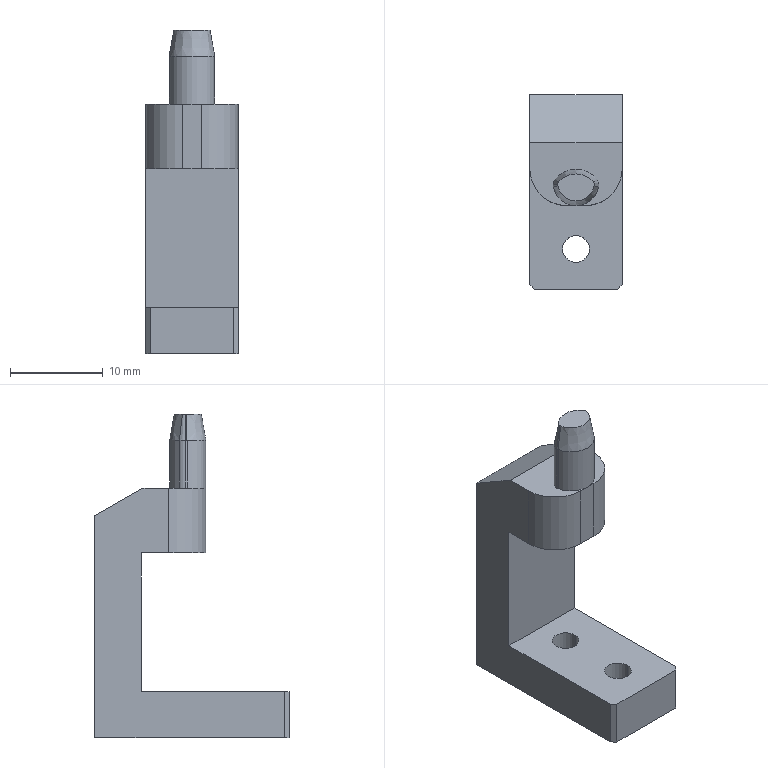Part | SolidWorks | features ICE 4, Chamfer 3, Fillet 2, Extrusion 1, HoleWzd 1 | 1 solid | 36 faces | box 10 x 21 x 35 mm | volume 2531 mm3 | plane 16 | cylinder 15 | cone 5 | commonest cylinder face diameters 2.9 x4 4 x4 2 x3 8 x2 5 x1 5.831 x1
STEP:
#1=CARTESIAN_POINT('',(2.,-11.65,-7.9));
#2=VERTEX_POINT('',#1);
#3=CARTESIAN_POINT('',(-2.,-11.65,-7.9));
#4=VERTEX_POINT('',#3);
#5=CARTESIAN_POINT('',(0.,-11.65,-7.9));
#6=DIRECTION('',(0.,0.,-1.));
#7=DIRECTION('',(-1.,0.,0.));
#8=AXIS2_PLACEMENT_3D('',#5,#6,#7);
#9=CIRCLE('',#8,2.);
#10=EDGE_CURVE('',#2,#4,#9,.T.);
#11=ORIENTED_EDGE('',*,*,#10,.F.);
#12=CARTESIAN_POINT('',(2.,-11.65,-10.));
#13=VERTEX_POINT('',#12);
#14=CARTESIAN_POINT('',(2.,-11.65,-7.9));
#15=DIRECTION('',(0.,0.,-1.));
#16=VECTOR('',#15,1000.);
#17=LINE('',#14,#16);
#18=EDGE_CURVE('',#2,#13,#17,.T.);
#19=ORIENTED_EDGE('',*,*,#18,.T.);
#20=CARTESIAN_POINT('',(-2.,-11.65,-10.));
#21=VERTEX_POINT('',#20);
#22=CARTESIAN_POINT('',(0.,-11.65,-10.));
#23=DIRECTION('',(0.,0.,-1.));
#24=DIRECTION('',(-1.,0.,0.));
#25=AXIS2_PLACEMENT_3D('',#22,#23,#24);
#26=CIRCLE('',#25,2.);
#27=EDGE_CURVE('',#13,#21,#26,.T.);
#28=ORIENTED_EDGE('',*,*,#27,.T.);
#29=CARTESIAN_POINT('',(-2.,-11.65,-7.9));
#30=DIRECTION('',(0.,0.,-1.));
#31=VECTOR('',#30,1000.);
#32=LINE('',#29,#31);
#33=EDGE_CURVE('',#4,#21,#32,.T.);
#34=ORIENTED_EDGE('',*,*,#33,.F.);
#35=EDGE_LOOP('',(#11,#19,#28,#34));
#36=FACE_OUTER_BOUND('',#35,.T.);
#37=CARTESIAN_POINT('',(0.,-11.65,-7.9));
#38=DIRECTION('',(0.,0.,-1.));
#39=DIRECTION('',(-1.,0.,0.));
#40=AXIS2_PLACEMENT_3D('',#37,#38,#39);
#41=CYLINDRICAL_SURFACE('',#40,2.);
#42=ADVANCED_FACE('',(#36),#41,.F.);
#43=CARTESIAN_POINT('',(2.,-3.65,-7.9));
#44=VERTEX_POINT('',#43);
#45=CARTESIAN_POINT('',(-2.,-3.65,-7.9));
#46=VERTEX_POINT('',#45);
#47=CARTESIAN_POINT('',(0.,-3.65,-7.9));
#48=DIRECTION('',(0.,0.,-1.));
#49=DIRECTION('',(-1.,0.,0.));
#50=AXIS2_PLACEMENT_3D('',#47,#48,#49);
#51=CIRCLE('',#50,2.);
#52=EDGE_CURVE('',#44,#46,#51,.T.);
#53=ORIENTED_EDGE('',*,*,#52,.F.);
#54=CARTESIAN_POINT('',(2.,-3.65,-10.));
#55=VERTEX_POINT('',#54);
#56=CARTESIAN_POINT('',(2.,-3.65,-7.9));
#57=DIRECTION('',(0.,0.,-1.));
#58=VECTOR('',#57,1000.);
#59=LINE('',#56,#58);
#60=EDGE_CURVE('',#44,#55,#59,.T.);
#61=ORIENTED_EDGE('',*,*,#60,.T.);
#62=CARTESIAN_POINT('',(-2.,-3.65,-10.));
#63=VERTEX_POINT('',#62);
#64=CARTESIAN_POINT('',(0.,-3.65,-10.));
#65=DIRECTION('',(0.,0.,-1.));
#66=DIRECTION('',(-1.,0.,0.));
#67=AXIS2_PLACEMENT_3D('',#64,#65,#66);
#68=CIRCLE('',#67,2.);
#69=EDGE_CURVE('',#55,#63,#68,.T.);
#70=ORIENTED_EDGE('',*,*,#69,.T.);
#71=CARTESIAN_POINT('',(-2.,-3.65,-7.9));
#72=DIRECTION('',(0.,0.,-1.));
#73=VECTOR('',#72,1000.);
#74=LINE('',#71,#73);
#75=EDGE_CURVE('',#46,#63,#74,.T.);
#76=ORIENTED_EDGE('',*,*,#75,.F.);
#77=EDGE_LOOP('',(#53,#61,#70,#76));
#78=FACE_OUTER_BOUND('',#77,.T.);
#79=CARTESIAN_POINT('',(0.,-3.65,-7.9));
#80=DIRECTION('',(0.,0.,-1.));
#81=DIRECTION('',(-1.,0.,0.));
#82=AXIS2_PLACEMENT_3D('',#79,#80,#81);
#83=CYLINDRICAL_SURFACE('',#82,2.);
#84=ADVANCED_FACE('',(#78),#83,.F.);
#85=CARTESIAN_POINT('',(-1.974,-4.777,25.));
#86=VERTEX_POINT('',#85);
#87=CARTESIAN_POINT('',(-1.966,-4.869,25.));
#88=VERTEX_POINT('',#87);
#89=CARTESIAN_POINT('',(-1.474,-4.777,25.));
#90=DIRECTION('',(0.,0.,1.));
#91=DIRECTION('',(-1.,0.,0.));
#92=AXIS2_PLACEMENT_3D('',#89,#90,#91);
#93=CIRCLE('',#92,0.5);
#94=EDGE_CURVE('',#86,#88,#93,.T.);
#95=ORIENTED_EDGE('',*,*,#94,.F.);
#96=CARTESIAN_POINT('',(-2.474,-4.777,22.164));
#97=VERTEX_POINT('',#96);
#98=CARTESIAN_POINT('',(-1.974,-4.777,25.));
#99=DIRECTION('',(-0.1736,0.,-0.9848));
#100=VECTOR('',#99,1000.);
#101=LINE('',#98,#100);
#102=EDGE_CURVE('',#86,#97,#101,.T.);
#103=ORIENTED_EDGE('',*,*,#102,.T.);
#104=CARTESIAN_POINT('',(-2.457,-4.962,22.164));
#105=VERTEX_POINT('',#104);
#106=CARTESIAN_POINT('',(-1.474,-4.777,22.164));
#107=DIRECTION('',(0.,0.,-1.));
#108=DIRECTION('',(-1.,0.,0.));
#109=AXIS2_PLACEMENT_3D('',#106,#107,#108);
#110=CIRCLE('',#109,1.);
#111=EDGE_CURVE('',#105,#97,#110,.T.);
#112=ORIENTED_EDGE('',*,*,#111,.F.);
#113=CARTESIAN_POINT('',(-2.457,-4.962,22.164));
#114=DIRECTION('',(0.1707,0.03207,0.9848));
#115=VECTOR('',#114,1000.);
#116=LINE('',#113,#115);
#117=EDGE_CURVE('',#105,#88,#116,.T.);
#118=ORIENTED_EDGE('',*,*,#117,.T.);
#119=EDGE_LOOP('',(#95,#103,#112,#118));
#120=FACE_OUTER_BOUND('',#119,.T.);
#121=CARTESIAN_POINT('',(-1.474,-4.777,25.));
#122=DIRECTION('',(0.,0.,-1.));
#123=DIRECTION('',(-1.,0.,0.));
#124=AXIS2_PLACEMENT_3D('',#121,#122,#123);
#125=CONICAL_SURFACE('',#124,0.5,0.1745);
#126=ADVANCED_FACE('',(#120),#125,.T.);
#127=ORIENTED_EDGE('',*,*,#111,.T.);
#128=CARTESIAN_POINT('',(-2.474,-4.777,17.));
#129=VERTEX_POINT('',#128);
#130=CARTESIAN_POINT('',(-2.474,-4.777,25.));
#131=DIRECTION('',(0.,0.,-1.));
#132=VECTOR('',#131,1000.);
#133=LINE('',#130,#132);
#134=EDGE_CURVE('',#97,#129,#133,.T.);
#135=ORIENTED_EDGE('',*,*,#134,.T.);
#136=CARTESIAN_POINT('',(-2.457,-4.962,17.));
#137=VERTEX_POINT('',#136);
#138=CARTESIAN_POINT('',(-1.474,-4.777,17.));
#139=DIRECTION('',(0.,0.,-1.));
#140=DIRECTION('',(1.,0.,0.));
#141=AXIS2_PLACEMENT_3D('',#138,#139,#140);
#142=CIRCLE('',#141,1.);
#143=EDGE_CURVE('',#137,#129,#142,.T.);
#144=ORIENTED_EDGE('',*,*,#143,.F.);
#145=CARTESIAN_POINT('',(-2.457,-4.962,25.));
#146=DIRECTION('',(0.,0.,-1.));
#147=VECTOR('',#146,1000.);
#148=LINE('',#145,#147);
#149=EDGE_CURVE('',#105,#137,#148,.T.);
#150=ORIENTED_EDGE('',*,*,#149,.F.);
#151=EDGE_LOOP('',(#127,#135,#144,#150));
#152=FACE_OUTER_BOUND('',#151,.T.);
#153=CARTESIAN_POINT('',(-1.474,-4.777,25.));
#154=DIRECTION('',(0.,0.,-1.));
#155=DIRECTION('',(-1.,0.,0.));
#156=AXIS2_PLACEMENT_3D('',#153,#154,#155);
#157=CYLINDRICAL_SURFACE('',#156,1.);
#158=ADVANCED_FACE('',(#152),#157,.T.);
#159=CARTESIAN_POINT('',(-1.45,-3.65,-7.9));
#160=VERTEX_POINT('',#159);
#161=CARTESIAN_POINT('',(1.45,-3.65,-7.9));
#162=VERTEX_POINT('',#161);
#163=CARTESIAN_POINT('',(0.,-3.65,-7.9));
#164=DIRECTION('',(0.,0.,1.));
#165=DIRECTION('',(-1.,0.,0.));
#166=AXIS2_PLACEMENT_3D('',#163,#164,#165);
#167=CIRCLE('',#166,1.45);
#168=EDGE_CURVE('',#160,#162,#167,.T.);
#169=ORIENTED_EDGE('',*,*,#168,.F.);
#170=CARTESIAN_POINT('',(-1.45,-3.65,-5.));
#171=VERTEX_POINT('',#170);
#172=CARTESIAN_POINT('',(-1.45,-3.65,-5.));
#173=DIRECTION('',(0.,0.,1.));
#174=VECTOR('',#173,1000.);
#175=LINE('',#172,#174);
#176=EDGE_CURVE('',#160,#171,#175,.T.);
#177=ORIENTED_EDGE('',*,*,#176,.T.);
#178=CARTESIAN_POINT('',(1.45,-3.65,-5.));
#179=VERTEX_POINT('',#178);
#180=CARTESIAN_POINT('',(0.,-3.65,-5.));
#181=DIRECTION('',(0.,0.,1.));
#182=DIRECTION('',(1.,0.,0.));
#183=AXIS2_PLACEMENT_3D('',#180,#181,#182);
#184=CIRCLE('',#183,1.45);
#185=EDGE_CURVE('',#171,#179,#184,.T.);
#186=ORIENTED_EDGE('',*,*,#185,.T.);
#187=CARTESIAN_POINT('',(1.45,-3.65,-5.));
#188=DIRECTION('',(0.,0.,1.));
#189=VECTOR('',#188,1000.);
#190=LINE('',#187,#189);
#191=EDGE_CURVE('',#162,#179,#190,.T.);
#192=ORIENTED_EDGE('',*,*,#191,.F.);
#193=EDGE_LOOP('',(#169,#177,#186,#192));
#194=FACE_OUTER_BOUND('',#193,.T.);
#195=CARTESIAN_POINT('',(0.,-3.65,-5.));
#196=DIRECTION('',(0.,0.,1.));
#197=DIRECTION('',(1.,0.,0.));
#198=AXIS2_PLACEMENT_3D('',#195,#196,#197);
#199=CYLINDRICAL_SURFACE('',#198,1.45);
#200=ADVANCED_FACE('',(#194),#199,.F.);
#201=CARTESIAN_POINT('',(-1.45,-11.65,-7.9));
#202=VERTEX_POINT('',#201);
#203=CARTESIAN_POINT('',(1.45,-11.65,-7.9));
#204=VERTEX_POINT('',#203);
#205=CARTESIAN_POINT('',(0.,-11.65,-7.9));
#206=DIRECTION('',(0.,0.,1.));
#207=DIRECTION('',(-1.,0.,0.));
#208=AXIS2_PLACEMENT_3D('',#205,#206,#207);
#209=CIRCLE('',#208,1.45);
#210=EDGE_CURVE('',#202,#204,#209,.T.);
#211=ORIENTED_EDGE('',*,*,#210,.F.);
#212=CARTESIAN_POINT('',(-1.45,-11.65,-5.));
#213=VERTEX_POINT('',#212);
#214=CARTESIAN_POINT('',(-1.45,-11.65,-5.));
#215=DIRECTION('',(0.,0.,1.));
#216=VECTOR('',#215,1000.);
#217=LINE('',#214,#216);
#218=EDGE_CURVE('',#202,#213,#217,.T.);
#219=ORIENTED_EDGE('',*,*,#218,.T.);
#220=CARTESIAN_POINT('',(1.45,-11.65,-5.));
#221=VERTEX_POINT('',#220);
#222=CARTESIAN_POINT('',(0.,-11.65,-5.));
#223=DIRECTION('',(0.,0.,1.));
#224=DIRECTION('',(1.,0.,0.));
#225=AXIS2_PLACEMENT_3D('',#222,#223,#224);
#226=CIRCLE('',#225,1.45);
#227=EDGE_CURVE('',#213,#221,#226,.T.);
#228=ORIENTED_EDGE('',*,*,#227,.T.);
#229=CARTESIAN_POINT('',(1.45,-11.65,-5.));
#230=DIRECTION('',(0.,0.,1.));
#231=VECTOR('',#230,1000.);
#232=LINE('',#229,#231);
#233=EDGE_CURVE('',#204,#221,#232,.T.);
#234=ORIENTED_EDGE('',*,*,#233,.F.);
#235=EDGE_LOOP('',(#211,#219,#228,#234));
#236=FACE_OUTER_BOUND('',#235,.T.);
#237=CARTESIAN_POINT('',(0.,-11.65,-5.));
#238=DIRECTION('',(0.,0.,1.));
#239=DIRECTION('',(1.,0.,0.));
#240=AXIS2_PLACEMENT_3D('',#237,#238,#239);
#241=CYLINDRICAL_SURFACE('',#240,1.45);
#242=ADVANCED_FACE('',(#236),#241,.F.);
#243=ORIENTED_EDGE('',*,*,#218,.F.);
#244=CARTESIAN_POINT('',(0.,-11.65,-7.9));
#245=DIRECTION('',(0.,0.,1.));
#246=DIRECTION('',(-1.,0.,0.));
#247=AXIS2_PLACEMENT_3D('',#244,#245,#246);
#248=CIRCLE('',#247,1.45);
#249=EDGE_CURVE('',#204,#202,#248,.T.);
#250=ORIENTED_EDGE('',*,*,#249,.F.);
#251=ORIENTED_EDGE('',*,*,#233,.T.);
#252=CARTESIAN_POINT('',(0.,-11.65,-5.));
#253=DIRECTION('',(0.,0.,1.));
#254=DIRECTION('',(1.,0.,0.));
#255=AXIS2_PLACEMENT_3D('',#252,#253,#254);
#256=CIRCLE('',#255,1.45);
#257=EDGE_CURVE('',#221,#213,#256,.T.);
#258=ORIENTED_EDGE('',*,*,#257,.T.);
#259=EDGE_LOOP('',(#243,#250,#251,#258));
#260=FACE_OUTER_BOUND('',#259,.T.);
#261=CARTESIAN_POINT('',(0.,-11.65,-5.));
#262=DIRECTION('',(0.,0.,1.));
#263=DIRECTION('',(1.,0.,0.));
#264=AXIS2_PLACEMENT_3D('',#261,#262,#263);
#265=CYLINDRICAL_SURFACE('',#264,1.45);
#266=ADVANCED_FACE('',(#260),#265,.F.);
#267=ORIENTED_EDGE('',*,*,#176,.F.);
#268=CARTESIAN_POINT('',(0.,-3.65,-7.9));
#269=DIRECTION('',(0.,0.,1.));
#270=DIRECTION('',(-1.,0.,0.));
#271=AXIS2_PLACEMENT_3D('',#268,#269,#270);
#272=CIRCLE('',#271,1.45);
#273=EDGE_CURVE('',#162,#160,#272,.T.);
#274=ORIENTED_EDGE('',*,*,#273,.F.);
#275=ORIENTED_EDGE('',*,*,#191,.T.);
#276=CARTESIAN_POINT('',(0.,-3.65,-5.));
#277=DIRECTION('',(0.,0.,1.));
#278=DIRECTION('',(1.,0.,0.));
#279=AXIS2_PLACEMENT_3D('',#276,#277,#278);
#280=CIRCLE('',#279,1.45);
#281=EDGE_CURVE('',#179,#171,#280,.T.);
#282=ORIENTED_EDGE('',*,*,#281,.T.);
#283=EDGE_LOOP('',(#267,#274,#275,#282));
#284=FACE_OUTER_BOUND('',#283,.T.);
#285=CARTESIAN_POINT('',(0.,-3.65,-5.));
#286=DIRECTION('',(0.,0.,1.));
#287=DIRECTION('',(1.,0.,0.));
#288=AXIS2_PLACEMENT_3D('',#285,#286,#287);
#289=CYLINDRICAL_SURFACE('',#288,1.45);
#290=ADVANCED_FACE('',(#284),#289,.F.);
#291=CARTESIAN_POINT('',(5.,-15.5,-5.));
#292=VERTEX_POINT('',#291);
#293=CARTESIAN_POINT('',(5.,0.,-5.));
#294=VERTEX_POINT('',#293);
#295=CARTESIAN_POINT('',(5.,-16.,-5.));
#296=DIRECTION('',(0.,1.,0.));
#297=VECTOR('',#296,1000.);
#298=LINE('',#295,#297);
#299=EDGE_CURVE('',#292,#294,#298,.T.);
#300=ORIENTED_EDGE('',*,*,#299,.F.);
#301=CARTESIAN_POINT('',(5.,-15.5,-10.));
#302=VERTEX_POINT('',#301);
#303=CARTESIAN_POINT('',(5.,-15.5,-10.));
#304=DIRECTION('',(0.,0.,-1.));
#305=VECTOR('',#304,1000.);
#306=LINE('',#303,#305);
#307=EDGE_CURVE('',#292,#302,#306,.T.);
#308=ORIENTED_EDGE('',*,*,#307,.T.);
#309=CARTESIAN_POINT('',(5.,5.,-10.));
#310=VERTEX_POINT('',#309);
#311=CARTESIAN_POINT('',(5.,5.,-10.));
#312=DIRECTION('',(0.,-1.,0.));
#313=VECTOR('',#312,1000.);
#314=LINE('',#311,#313);
#315=EDGE_CURVE('',#310,#302,#314,.T.);
#316=ORIENTED_EDGE('',*,*,#315,.F.);
#317=CARTESIAN_POINT('',(5.,5.,14.));
#318=VERTEX_POINT('',#317);
#319=CARTESIAN_POINT('',(5.,5.,10.));
#320=DIRECTION('',(0.,0.,-1.));
#321=VECTOR('',#320,1000.);
#322=LINE('',#319,#321);
#323=EDGE_CURVE('',#318,#310,#322,.T.);
#324=ORIENTED_EDGE('',*,*,#323,.F.);
#325=CARTESIAN_POINT('',(5.,-0.1962,17.));
#326=VERTEX_POINT('',#325);
#327=CARTESIAN_POINT('',(5.,-0.1962,17.));
#328=DIRECTION('',(0.,-0.866,0.5));
#329=VECTOR('',#328,1000.);
#330=LINE('',#327,#329);
#331=EDGE_CURVE('',#318,#326,#330,.T.);
#332=ORIENTED_EDGE('',*,*,#331,.T.);
#333=CARTESIAN_POINT('',(5.,-3.,17.));
#334=VERTEX_POINT('',#333);
#335=CARTESIAN_POINT('',(5.,5.,17.));
#336=DIRECTION('',(0.,1.,0.));
#337=VECTOR('',#336,1000.);
#338=LINE('',#335,#337);
#339=EDGE_CURVE('',#334,#326,#338,.T.);
#340=ORIENTED_EDGE('',*,*,#339,.F.);
#341=CARTESIAN_POINT('',(5.,-3.,10.));
#342=VERTEX_POINT('',#341);
#343=CARTESIAN_POINT('',(5.,-3.,10.));
#344=DIRECTION('',(0.,0.,-1.));
#345=VECTOR('',#344,1000.);
#346=LINE('',#343,#345);
#347=EDGE_CURVE('',#334,#342,#346,.T.);
#348=ORIENTED_EDGE('',*,*,#347,.T.);
#349=CARTESIAN_POINT('',(5.,0.,10.));
#350=VERTEX_POINT('',#349);
#351=CARTESIAN_POINT('',(5.,5.,10.));
#352=DIRECTION('',(0.,1.,0.));
#353=VECTOR('',#352,1000.);
#354=LINE('',#351,#353);
#355=EDGE_CURVE('',#342,#350,#354,.T.);
#356=ORIENTED_EDGE('',*,*,#355,.T.);
#357=CARTESIAN_POINT('',(5.,0.,10.));
#358=DIRECTION('',(0.,0.,-1.));
#359=VECTOR('',#358,1000.);
#360=LINE('',#357,#359);
#361=EDGE_CURVE('',#350,#294,#360,.T.);
#362=ORIENTED_EDGE('',*,*,#361,.T.);
#363=EDGE_LOOP('',(#300,#308,#316,#324,#332,#340,#348,#356,#362));
#364=FACE_OUTER_BOUND('',#363,.T.);
#365=CARTESIAN_POINT('',(5.,5.,10.));
#366=DIRECTION('',(-1.,0.,0.));
#367=DIRECTION('',(0.,0.,1.));
#368=AXIS2_PLACEMENT_3D('',#365,#366,#367);
#369=PLANE('',#368);
#370=ADVANCED_FACE('',(#364),#369,.F.);
#371=CARTESIAN_POINT('',(0.,-11.65,-10.));
#372=DIRECTION('',(0.,0.,-1.));
#373=DIRECTION('',(-1.,0.,0.));
#374=AXIS2_PLACEMENT_3D('',#371,#372,#373);
#375=CIRCLE('',#374,2.);
#376=EDGE_CURVE('',#21,#13,#375,.T.);
#377=ORIENTED_EDGE('',*,*,#376,.F.);
#378=ORIENTED_EDGE('',*,*,#27,.F.);
#379=EDGE_LOOP('',(#377,#378));
#380=FACE_BOUND('',#379,.T.);
#381=CARTESIAN_POINT('',(0.,-3.65,-10.));
#382=DIRECTION('',(0.,0.,-1.));
#383=DIRECTION('',(-1.,0.,0.));
#384=AXIS2_PLACEMENT_3D('',#381,#382,#383);
#385=CIRCLE('',#384,2.);
#386=EDGE_CURVE('',#63,#55,#385,.T.);
#387=ORIENTED_EDGE('',*,*,#386,.F.);
#388=ORIENTED_EDGE('',*,*,#69,.F.);
#389=EDGE_LOOP('',(#387,#388));
#390=FACE_BOUND('',#389,.T.);
#391=ORIENTED_EDGE('',*,*,#315,.T.);
#392=CARTESIAN_POINT('',(4.5,-16.,-10.));
#393=VERTEX_POINT('',#392);
#394=CARTESIAN_POINT('',(4.5,-16.,-10.));
#395=DIRECTION('',(-0.7071,-0.7071,0.));
#396=VECTOR('',#395,1000.);
#397=LINE('',#394,#396);
#398=EDGE_CURVE('',#302,#393,#397,.T.);
#399=ORIENTED_EDGE('',*,*,#398,.T.);
#400=CARTESIAN_POINT('',(-4.5,-16.,-10.));
#401=VERTEX_POINT('',#400);
#402=CARTESIAN_POINT('',(5.,-16.,-10.));
#403=DIRECTION('',(1.,0.,0.));
#404=VECTOR('',#403,1000.);
#405=LINE('',#402,#404);
#406=EDGE_CURVE('',#401,#393,#405,.T.);
#407=ORIENTED_EDGE('',*,*,#406,.F.);
#408=CARTESIAN_POINT('',(-5.,-15.5,-10.));
#409=VERTEX_POINT('',#408);
#410=CARTESIAN_POINT('',(-4.5,-16.,-10.));
#411=DIRECTION('',(-0.7071,0.7071,0.));
#412=VECTOR('',#411,1000.);
#413=LINE('',#410,#412);
#414=EDGE_CURVE('',#401,#409,#413,.T.);
#415=ORIENTED_EDGE('',*,*,#414,.T.);
#416=CARTESIAN_POINT('',(-5.,5.,-10.));
#417=VERTEX_POINT('',#416);
#418=CARTESIAN_POINT('',(-5.,5.,-10.));
#419=DIRECTION('',(0.,-1.,0.));
#420=VECTOR('',#419,1000.);
#421=LINE('',#418,#420);
#422=EDGE_CURVE('',#417,#409,#421,.T.);
#423=ORIENTED_EDGE('',*,*,#422,.F.);
#424=CARTESIAN_POINT('',(-5.,5.,-10.));
#425=DIRECTION('',(-1.,0.,0.));
#426=VECTOR('',#425,1000.);
#427=LINE('',#424,#426);
#428=EDGE_CURVE('',#310,#417,#427,.T.);
#429=ORIENTED_EDGE('',*,*,#428,.F.);
#430=EDGE_LOOP('',(#391,#399,#407,#415,#423,#429));
#431=FACE_OUTER_BOUND('',#430,.T.);
#432=CARTESIAN_POINT('',(-5.,5.,-10.));
#433=DIRECTION('',(0.,0.,1.));
#434=DIRECTION('',(1.,0.,0.));
#435=AXIS2_PLACEMENT_3D('',#432,#433,#434);
#436=PLANE('',#435);
#437=ADVANCED_FACE('',(#380,#390,#431),#436,.F.);
#438=ORIENTED_EDGE('',*,*,#422,.T.);
#439=CARTESIAN_POINT('',(-5.,-15.5,-5.));
#440=VERTEX_POINT('',#439);
#441=CARTESIAN_POINT('',(-5.,-15.5,-5.));
#442=DIRECTION('',(0.,0.,1.));
#443=VECTOR('',#442,1000.);
#444=LINE('',#441,#443);
#445=EDGE_CURVE('',#409,#440,#444,.T.);
#446=ORIENTED_EDGE('',*,*,#445,.T.);
#447=CARTESIAN_POINT('',(-5.,0.,-5.));
#448=VERTEX_POINT('',#447);
#449=CARTESIAN_POINT('',(-5.,-16.,-5.));
#450=DIRECTION('',(0.,1.,0.));
#451=VECTOR('',#450,1000.);
#452=LINE('',#449,#451);
#453=EDGE_CURVE('',#440,#448,#452,.T.);
#454=ORIENTED_EDGE('',*,*,#453,.T.);
#455=CARTESIAN_POINT('',(-5.,0.,10.));
#456=VERTEX_POINT('',#455);
#457=CARTESIAN_POINT('',(-5.,0.,10.));
#458=DIRECTION('',(0.,0.,1.));
#459=VECTOR('',#458,1000.);
#460=LINE('',#457,#459);
#461=EDGE_CURVE('',#448,#456,#460,.T.);
#462=ORIENTED_EDGE('',*,*,#461,.T.);
#463=CARTESIAN_POINT('',(-5.,-3.,10.));
#464=VERTEX_POINT('',#463);
#465=CARTESIAN_POINT('',(-5.,5.,10.));
#466=DIRECTION('',(0.,-1.,0.));
#467=VECTOR('',#466,1000.);
#468=LINE('',#465,#467);
#469=EDGE_CURVE('',#456,#464,#468,.T.);
#470=ORIENTED_EDGE('',*,*,#469,.T.);
#471=CARTESIAN_POINT('',(-5.,-3.,17.));
#472=VERTEX_POINT('',#471);
#473=CARTESIAN_POINT('',(-5.,-3.,10.));
#474=DIRECTION('',(0.,0.,1.));
#475=VECTOR('',#474,1000.);
#476=LINE('',#473,#475);
#477=EDGE_CURVE('',#464,#472,#476,.T.);
#478=ORIENTED_EDGE('',*,*,#477,.T.);
#479=CARTESIAN_POINT('',(-5.,-0.1962,17.));
#480=VERTEX_POINT('',#479);
#481=CARTESIAN_POINT('',(-5.,5.,17.));
#482=DIRECTION('',(0.,-1.,0.));
#483=VECTOR('',#482,1000.);
#484=LINE('',#481,#483);
#485=EDGE_CURVE('',#480,#472,#484,.T.);
#486=ORIENTED_EDGE('',*,*,#485,.F.);
#487=CARTESIAN_POINT('',(-5.,5.,14.));
#488=VERTEX_POINT('',#487);
#489=CARTESIAN_POINT('',(-5.,-0.1962,17.));
#490=DIRECTION('',(0.,0.866,-0.5));
#491=VECTOR('',#490,1000.);
#492=LINE('',#489,#491);
#493=EDGE_CURVE('',#480,#488,#492,.T.);
#494=ORIENTED_EDGE('',*,*,#493,.T.);
#495=CARTESIAN_POINT('',(-5.,5.,10.));
#496=DIRECTION('',(0.,0.,1.));
#497=VECTOR('',#496,1000.);
#498=LINE('',#495,#497);
#499=EDGE_CURVE('',#417,#488,#498,.T.);
#500=ORIENTED_EDGE('',*,*,#499,.F.);
#501=EDGE_LOOP('',(#438,#446,#454,#462,#470,#478,#486,#494,#500));
#502=FACE_OUTER_BOUND('',#501,.T.);
#503=CARTESIAN_POINT('',(-5.,5.,10.));
#504=DIRECTION('',(1.,0.,0.));
#505=DIRECTION('',(0.,0.,-1.));
#506=AXIS2_PLACEMENT_3D('',#503,#504,#505);
#507=PLANE('',#506);
#508=ADVANCED_FACE('',(#502),#507,.F.);
#509=ORIENTED_EDGE('',*,*,#499,.T.);
#510=CARTESIAN_POINT('',(5.,5.,14.));
#511=DIRECTION('',(1.,0.,0.));
#512=VECTOR('',#511,1000.);
#513=LINE('',#510,#512);
#514=EDGE_CURVE('',#488,#318,#513,.T.);
#515=ORIENTED_EDGE('',*,*,#514,.T.);
#516=ORIENTED_EDGE('',*,*,#323,.T.);
#517=ORIENTED_EDGE('',*,*,#428,.T.);
#518=EDGE_LOOP('',(#509,#515,#516,#517));
#519=FACE_OUTER_BOUND('',#518,.T.);
#520=CARTESIAN_POINT('',(0.,5.,0.));
#521=DIRECTION('',(0.,-1.,0.));
#522=DIRECTION('',(0.,0.,-1.));
#523=AXIS2_PLACEMENT_3D('',#520,#521,#522);
#524=PLANE('',#523);
#525=ADVANCED_FACE('',(#519),#524,.F.);
#526=CARTESIAN_POINT('',(5.,0.,-5.));
#527=DIRECTION('',(-1.,0.,0.));
#528=VECTOR('',#527,1000.);
#529=LINE('',#526,#528);
#530=EDGE_CURVE('',#294,#448,#529,.T.);
#531=ORIENTED_EDGE('',*,*,#530,.F.);
#532=ORIENTED_EDGE('',*,*,#361,.F.);
#533=CARTESIAN_POINT('',(-5.,0.,10.));
#534=DIRECTION('',(1.,0.,0.));
#535=VECTOR('',#534,1000.);
#536=LINE('',#533,#535);
#537=EDGE_CURVE('',#456,#350,#536,.T.);
#538=ORIENTED_EDGE('',*,*,#537,.F.);
#539=ORIENTED_EDGE('',*,*,#461,.F.);
#540=EDGE_LOOP('',(#531,#532,#538,#539));
#541=FACE_OUTER_BOUND('',#540,.T.);
#542=CARTESIAN_POINT('',(0.,0.,0.));
#543=DIRECTION('',(0.,-1.,0.));
#544=DIRECTION('',(0.,0.,-1.));
#545=AXIS2_PLACEMENT_3D('',#542,#543,#544);
#546=PLANE('',#545);
#547=ADVANCED_FACE('',(#541),#546,.T.);
#548=ORIENTED_EDGE('',*,*,#257,.F.);
#549=ORIENTED_EDGE('',*,*,#227,.F.);
#550=EDGE_LOOP('',(#548,#549));
#551=FACE_BOUND('',#550,.T.);
#552=ORIENTED_EDGE('',*,*,#281,.F.);
#553=ORIENTED_EDGE('',*,*,#185,.F.);
#554=EDGE_LOOP('',(#552,#553));
#555=FACE_BOUND('',#554,.T.);
#556=CARTESIAN_POINT('',(4.5,-16.,-5.));
#557=VERTEX_POINT('',#556);
#558=CARTESIAN_POINT('',(-4.5,-16.,-5.));
#559=VERTEX_POINT('',#558);
#560=CARTESIAN_POINT('',(5.,-16.,-5.));
#561=DIRECTION('',(-1.,0.,0.));
#562=VECTOR('',#561,1000.);
#563=LINE('',#560,#562);
#564=EDGE_CURVE('',#557,#559,#563,.T.);
#565=ORIENTED_EDGE('',*,*,#564,.F.);
#566=CARTESIAN_POINT('',(4.5,-16.,-5.));
#567=DIRECTION('',(0.7071,0.7071,0.));
#568=VECTOR('',#567,1000.);
#569=LINE('',#566,#568);
#570=EDGE_CURVE('',#557,#292,#569,.T.);
#571=ORIENTED_EDGE('',*,*,#570,.T.);
#572=ORIENTED_EDGE('',*,*,#299,.T.);
#573=ORIENTED_EDGE('',*,*,#530,.T.);
#574=ORIENTED_EDGE('',*,*,#453,.F.);
#575=CARTESIAN_POINT('',(-4.5,-16.,-5.));
#576=DIRECTION('',(0.7071,-0.7071,0.));
#577=VECTOR('',#576,1000.);
#578=LINE('',#575,#577);
#579=EDGE_CURVE('',#440,#559,#578,.T.);
#580=ORIENTED_EDGE('',*,*,#579,.T.);
#581=EDGE_LOOP('',(#565,#571,#572,#573,#574,#580));
#582=FACE_OUTER_BOUND('',#581,.T.);
#583=CARTESIAN_POINT('',(5.,-16.,-5.));
#584=DIRECTION('',(0.,0.,-1.));
#585=DIRECTION('',(-1.,0.,0.));
#586=AXIS2_PLACEMENT_3D('',#583,#584,#585);
#587=PLANE('',#586);
#588=ADVANCED_FACE('',(#551,#555,#582),#587,.F.);
#589=ORIENTED_EDGE('',*,*,#406,.T.);
#590=CARTESIAN_POINT('',(4.5,-16.,-5.));
#591=DIRECTION('',(0.,0.,1.));
#592=VECTOR('',#591,1000.);
#593=LINE('',#590,#592);
#594=EDGE_CURVE('',#393,#557,#593,.T.);
#595=ORIENTED_EDGE('',*,*,#594,.T.);
#596=ORIENTED_EDGE('',*,*,#564,.T.);
#597=CARTESIAN_POINT('',(-4.5,-16.,-10.));
#598=DIRECTION('',(0.,0.,-1.));
#599=VECTOR('',#598,1000.);
#600=LINE('',#597,#599);
#601=EDGE_CURVE('',#559,#401,#600,.T.);
#602=ORIENTED_EDGE('',*,*,#601,.T.);
#603=EDGE_LOOP('',(#589,#595,#596,#602));
#604=FACE_OUTER_BOUND('',#603,.T.);
#605=CARTESIAN_POINT('',(0.,-16.,0.));
#606=DIRECTION('',(0.,-1.,0.));
#607=DIRECTION('',(0.,0.,-1.));
#608=AXIS2_PLACEMENT_3D('',#605,#606,#607);
#609=PLANE('',#608);
#610=ADVANCED_FACE('',(#604),#609,.T.);
#611=ORIENTED_EDGE('',*,*,#355,.F.);
#612=CARTESIAN_POINT('',(1.,-7.,10.));
#613=VERTEX_POINT('',#612);
#614=CARTESIAN_POINT('',(1.,-3.,10.));
#615=DIRECTION('',(0.,0.,-1.));
#616=DIRECTION('',(1.,0.,0.));
#617=AXIS2_PLACEMENT_3D('',#614,#615,#616);
#618=CIRCLE('',#617,4.);
#619=EDGE_CURVE('',#342,#613,#618,.T.);
#620=ORIENTED_EDGE('',*,*,#619,.T.);
#621=CARTESIAN_POINT('',(-1.,-7.,10.));
#622=VERTEX_POINT('',#621);
#623=CARTESIAN_POINT('',(-5.,-7.,10.));
#624=DIRECTION('',(1.,0.,0.));
#625=VECTOR('',#624,1000.);
#626=LINE('',#623,#625);
#627=EDGE_CURVE('',#622,#613,#626,.T.);
#628=ORIENTED_EDGE('',*,*,#627,.F.);
#629=CARTESIAN_POINT('',(-1.,-3.,10.));
#630=DIRECTION('',(0.,0.,-1.));
#631=DIRECTION('',(1.,0.,0.));
#632=AXIS2_PLACEMENT_3D('',#629,#630,#631);
#633=CIRCLE('',#632,4.);
#634=EDGE_CURVE('',#622,#464,#633,.T.);
#635=ORIENTED_EDGE('',*,*,#634,.T.);
#636=ORIENTED_EDGE('',*,*,#469,.F.);
#637=ORIENTED_EDGE('',*,*,#537,.T.);
#638=EDGE_LOOP('',(#611,#620,#628,#635,#636,#637));
#639=FACE_OUTER_BOUND('',#638,.T.);
#640=CARTESIAN_POINT('',(0.,0.,10.));
#641=DIRECTION('',(0.,0.,1.));
#642=DIRECTION('',(1.,0.,0.));
#643=AXIS2_PLACEMENT_3D('',#640,#641,#642);
#644=PLANE('',#643);
#645=ADVANCED_FACE('',(#639),#644,.F.);
#646=ORIENTED_EDGE('',*,*,#627,.T.);
#647=CARTESIAN_POINT('',(1.,-7.,17.));
#648=VERTEX_POINT('',#647);
#649=CARTESIAN_POINT('',(1.,-7.,17.));
#650=DIRECTION('',(0.,0.,1.));
#651=VECTOR('',#650,1000.);
#652=LINE('',#649,#651);
#653=EDGE_CURVE('',#613,#648,#652,.T.);
#654=ORIENTED_EDGE('',*,*,#653,.T.);
#655=CARTESIAN_POINT('',(0.,-7.,17.));
#656=VERTEX_POINT('',#655);
#657=CARTESIAN_POINT('',(-5.,-7.,17.));
#658=DIRECTION('',(1.,0.,0.));
#659=VECTOR('',#658,1000.);
#660=LINE('',#657,#659);
#661=EDGE_CURVE('',#656,#648,#660,.T.);
#662=ORIENTED_EDGE('',*,*,#661,.F.);
#663=CARTESIAN_POINT('',(-1.,-7.,17.));
#664=VERTEX_POINT('',#663);
#665=CARTESIAN_POINT('',(-5.,-7.,17.));
#666=DIRECTION('',(1.,0.,0.));
#667=VECTOR('',#666,1000.);
#668=LINE('',#665,#667);
#669=EDGE_CURVE('',#664,#656,#668,.T.);
#670=ORIENTED_EDGE('',*,*,#669,.F.);
#671=CARTESIAN_POINT('',(-1.,-7.,17.));
#672=DIRECTION('',(0.,0.,-1.));
#673=VECTOR('',#672,1000.);
#674=LINE('',#671,#673);
#675=EDGE_CURVE('',#664,#622,#674,.T.);
#676=ORIENTED_EDGE('',*,*,#675,.T.);
#677=EDGE_LOOP('',(#646,#654,#662,#670,#676));
#678=FACE_OUTER_BOUND('',#677,.T.);
#679=CARTESIAN_POINT('',(-5.,-7.,17.));
#680=DIRECTION('',(0.,1.,0.));
#681=DIRECTION('',(0.,0.,1.));
#682=AXIS2_PLACEMENT_3D('',#679,#680,#681);
#683=PLANE('',#682);
#684=ADVANCED_FACE('',(#678),#683,.F.);
#685=CARTESIAN_POINT('',(2.244,-4.138,17.));
#686=VERTEX_POINT('',#685);
#687=CARTESIAN_POINT('',(-2.244,-4.138,17.));
#688=VERTEX_POINT('',#687);
#689=CARTESIAN_POINT('',(0.,-6.,17.));
#690=DIRECTION('',(0.,0.,1.));
#691=DIRECTION('',(-1.,0.,0.));
#692=AXIS2_PLACEMENT_3D('',#689,#690,#691);
#693=CIRCLE('',#692,2.915);
#694=EDGE_CURVE('',#686,#688,#693,.T.);
#695=ORIENTED_EDGE('',*,*,#694,.F.);
#696=CARTESIAN_POINT('',(2.457,-4.962,17.));
#697=VERTEX_POINT('',#696);
#698=CARTESIAN_POINT('',(1.474,-4.777,17.));
#699=DIRECTION('',(0.,0.,-1.));
#700=DIRECTION('',(1.,0.,0.));
#701=AXIS2_PLACEMENT_3D('',#698,#699,#700);
#702=CIRCLE('',#701,1.);
#703=EDGE_CURVE('',#686,#697,#702,.T.);
#704=ORIENTED_EDGE('',*,*,#703,.T.);
#705=CARTESIAN_POINT('',(0.,-4.5,17.));
#706=DIRECTION('',(0.,0.,1.));
#707=DIRECTION('',(1.,0.,0.));
#708=AXIS2_PLACEMENT_3D('',#705,#706,#707);
#709=CIRCLE('',#708,2.5);
#710=EDGE_CURVE('',#656,#697,#709,.T.);
#711=ORIENTED_EDGE('',*,*,#710,.F.);
#712=ORIENTED_EDGE('',*,*,#661,.T.);
#713=CARTESIAN_POINT('',(1.,-3.,17.));
#714=DIRECTION('',(0.,0.,1.));
#715=DIRECTION('',(1.,0.,0.));
#716=AXIS2_PLACEMENT_3D('',#713,#714,#715);
#717=CIRCLE('',#716,4.);
#718=EDGE_CURVE('',#648,#334,#717,.T.);
#719=ORIENTED_EDGE('',*,*,#718,.T.);
#720=ORIENTED_EDGE('',*,*,#339,.T.);
#721=CARTESIAN_POINT('',(-5.,-0.1962,17.));
#722=DIRECTION('',(-1.,0.,0.));
#723=VECTOR('',#722,1000.);
#724=LINE('',#721,#723);
#725=EDGE_CURVE('',#326,#480,#724,.T.);
#726=ORIENTED_EDGE('',*,*,#725,.T.);
#727=ORIENTED_EDGE('',*,*,#485,.T.);
#728=CARTESIAN_POINT('',(-1.,-3.,17.));
#729=DIRECTION('',(0.,0.,1.));
#730=DIRECTION('',(1.,0.,0.));
#731=AXIS2_PLACEMENT_3D('',#728,#729,#730);
#732=CIRCLE('',#731,4.);
#733=EDGE_CURVE('',#472,#664,#732,.T.);
#734=ORIENTED_EDGE('',*,*,#733,.T.);
#735=ORIENTED_EDGE('',*,*,#669,.T.);
#736=CARTESIAN_POINT('',(0.,-4.5,17.));
#737=DIRECTION('',(0.,0.,1.));
#738=DIRECTION('',(1.,0.,0.));
#739=AXIS2_PLACEMENT_3D('',#736,#737,#738);
#740=CIRCLE('',#739,2.5);
#741=EDGE_CURVE('',#137,#656,#740,.T.);
#742=ORIENTED_EDGE('',*,*,#741,.F.);
#743=ORIENTED_EDGE('',*,*,#143,.T.);
#744=CARTESIAN_POINT('',(-1.474,-4.777,17.));
#745=DIRECTION('',(0.,0.,-1.));
#746=DIRECTION('',(1.,0.,0.));
#747=AXIS2_PLACEMENT_3D('',#744,#745,#746);
#748=CIRCLE('',#747,1.);
#749=EDGE_CURVE('',#129,#688,#748,.T.);
#750=ORIENTED_EDGE('',*,*,#749,.T.);
#751=EDGE_LOOP('',(#695,#704,#711,#712,#719,#720,#726,#727,#734,#735,#742,#743,#750));
#752=FACE_OUTER_BOUND('',#751,.T.);
#753=CARTESIAN_POINT('',(0.,0.,17.));
#754=DIRECTION('',(0.,0.,1.));
#755=DIRECTION('',(1.,0.,0.));
#756=AXIS2_PLACEMENT_3D('',#753,#754,#755);
#757=PLANE('',#756);
#758=ADVANCED_FACE('',(#752),#757,.T.);
#759=ORIENTED_EDGE('',*,*,#331,.F.);
#760=ORIENTED_EDGE('',*,*,#514,.F.);
#761=ORIENTED_EDGE('',*,*,#493,.F.);
#762=ORIENTED_EDGE('',*,*,#725,.F.);
#763=EDGE_LOOP('',(#759,#760,#761,#762));
#764=FACE_OUTER_BOUND('',#763,.T.);
#765=CARTESIAN_POINT('',(0.,-0.1962,17.));
#766=DIRECTION('',(0.,0.5,0.866));
#767=DIRECTION('',(1.,0.,0.));
#768=AXIS2_PLACEMENT_3D('',#765,#766,#767);
#769=PLANE('',#768);
#770=ADVANCED_FACE('',(#764),#769,.T.);
#771=ORIENTED_EDGE('',*,*,#718,.F.);
#772=ORIENTED_EDGE('',*,*,#653,.F.);
#773=ORIENTED_EDGE('',*,*,#619,.F.);
#774=ORIENTED_EDGE('',*,*,#347,.F.);
#775=EDGE_LOOP('',(#771,#772,#773,#774));
#776=FACE_OUTER_BOUND('',#775,.T.);
#777=CARTESIAN_POINT('',(1.,-3.,10.));
#778=DIRECTION('',(0.,0.,-1.));
#779=DIRECTION('',(-1.,0.,0.));
#780=AXIS2_PLACEMENT_3D('',#777,#778,#779);
#781=CYLINDRICAL_SURFACE('',#780,4.);
#782=ADVANCED_FACE('',(#776),#781,.T.);
#783=ORIENTED_EDGE('',*,*,#733,.F.);
#784=ORIENTED_EDGE('',*,*,#477,.F.);
#785=ORIENTED_EDGE('',*,*,#634,.F.);
#786=ORIENTED_EDGE('',*,*,#675,.F.);
#787=EDGE_LOOP('',(#783,#784,#785,#786));
#788=FACE_OUTER_BOUND('',#787,.T.);
#789=CARTESIAN_POINT('',(-1.,-3.,17.));
#790=DIRECTION('',(0.,0.,-1.));
#791=DIRECTION('',(-1.,0.,0.));
#792=AXIS2_PLACEMENT_3D('',#789,#790,#791);
#793=CYLINDRICAL_SURFACE('',#792,4.);
#794=ADVANCED_FACE('',(#788),#793,.T.);
#795=ORIENTED_EDGE('',*,*,#398,.F.);
#796=ORIENTED_EDGE('',*,*,#307,.F.);
#797=ORIENTED_EDGE('',*,*,#570,.F.);
#798=ORIENTED_EDGE('',*,*,#594,.F.);
#799=EDGE_LOOP('',(#795,#796,#797,#798));
#800=FACE_OUTER_BOUND('',#799,.T.);
#801=CARTESIAN_POINT('',(4.5,-16.,0.));
#802=DIRECTION('',(0.7071,-0.7071,0.));
#803=DIRECTION('',(0.,0.,-1.));
#804=AXIS2_PLACEMENT_3D('',#801,#802,#803);
#805=PLANE('',#804);
#806=ADVANCED_FACE('',(#800),#805,.T.);
#807=ORIENTED_EDGE('',*,*,#579,.F.);
#808=ORIENTED_EDGE('',*,*,#445,.F.);
#809=ORIENTED_EDGE('',*,*,#414,.F.);
#810=ORIENTED_EDGE('',*,*,#601,.F.);
#811=EDGE_LOOP('',(#807,#808,#809,#810));
#812=FACE_OUTER_BOUND('',#811,.T.);
#813=CARTESIAN_POINT('',(-4.5,-16.,0.));
#814=DIRECTION('',(-0.7071,-0.7071,0.));
#815=DIRECTION('',(0.,0.,1.));
#816=AXIS2_PLACEMENT_3D('',#813,#814,#815);
#817=PLANE('',#816);
#818=ADVANCED_FACE('',(#812),#817,.T.);
#819=CARTESIAN_POINT('',(-2.244,-4.138,22.164));
#820=VERTEX_POINT('',#819);
#821=CARTESIAN_POINT('',(-2.244,-4.138,25.));
#822=DIRECTION('',(0.,0.,1.));
#823=VECTOR('',#822,1000.);
#824=LINE('',#821,#823);
#825=EDGE_CURVE('',#688,#820,#824,.T.);
#826=ORIENTED_EDGE('',*,*,#825,.T.);
#827=CARTESIAN_POINT('',(2.244,-4.138,22.164));
#828=VERTEX_POINT('',#827);
#829=CARTESIAN_POINT('',(0.,-6.,22.164));
#830=DIRECTION('',(0.,0.,-1.));
#831=DIRECTION('',(-1.,0.,0.));
#832=AXIS2_PLACEMENT_3D('',#829,#830,#831);
#833=CIRCLE('',#832,2.915);
#834=EDGE_CURVE('',#820,#828,#833,.T.);
#835=ORIENTED_EDGE('',*,*,#834,.T.);
#836=CARTESIAN_POINT('',(2.244,-4.138,25.));
#837=DIRECTION('',(0.,0.,-1.));
#838=VECTOR('',#837,1000.);
#839=LINE('',#836,#838);
#840=EDGE_CURVE('',#828,#686,#839,.T.);
#841=ORIENTED_EDGE('',*,*,#840,.T.);
#842=ORIENTED_EDGE('',*,*,#694,.T.);
#843=EDGE_LOOP('',(#826,#835,#841,#842));
#844=FACE_OUTER_BOUND('',#843,.T.);
#845=CARTESIAN_POINT('',(0.,-6.,25.));
#846=DIRECTION('',(0.,0.,-1.));
#847=DIRECTION('',(-1.,0.,0.));
#848=AXIS2_PLACEMENT_3D('',#845,#846,#847);
#849=CYLINDRICAL_SURFACE('',#848,2.915);
#850=ADVANCED_FACE('',(#844),#849,.T.);
#851=CARTESIAN_POINT('',(2.457,-4.962,22.164));
#852=VERTEX_POINT('',#851);
#853=CARTESIAN_POINT('',(2.457,-4.962,25.));
#854=DIRECTION('',(0.,0.,1.));
#855=VECTOR('',#854,1000.);
#856=LINE('',#853,#855);
#857=EDGE_CURVE('',#697,#852,#856,.T.);
#858=ORIENTED_EDGE('',*,*,#857,.T.);
#859=CARTESIAN_POINT('',(0.,-4.5,22.164));
#860=DIRECTION('',(0.,0.,-1.));
#861=DIRECTION('',(-1.,0.,0.));
#862=AXIS2_PLACEMENT_3D('',#859,#860,#861);
#863=CIRCLE('',#862,2.5);
#864=EDGE_CURVE('',#852,#105,#863,.T.);
#865=ORIENTED_EDGE('',*,*,#864,.T.);
#866=ORIENTED_EDGE('',*,*,#149,.T.);
#867=ORIENTED_EDGE('',*,*,#741,.T.);
#868=ORIENTED_EDGE('',*,*,#710,.T.);
#869=EDGE_LOOP('',(#858,#865,#866,#867,#868));
#870=FACE_OUTER_BOUND('',#869,.T.);
#871=CARTESIAN_POINT('',(0.,-4.5,25.));
#872=DIRECTION('',(0.,0.,-1.));
#873=DIRECTION('',(-1.,0.,0.));
#874=AXIS2_PLACEMENT_3D('',#871,#872,#873);
#875=CYLINDRICAL_SURFACE('',#874,2.5);
#876=ADVANCED_FACE('',(#870),#875,.T.);
#877=CARTESIAN_POINT('',(1.966,-4.869,25.));
#878=VERTEX_POINT('',#877);
#879=CARTESIAN_POINT('',(1.859,-4.458,25.));
#880=VERTEX_POINT('',#879);
#881=CARTESIAN_POINT('',(1.474,-4.777,25.));
#882=DIRECTION('',(0.,0.,1.));
#883=DIRECTION('',(-1.,0.,0.));
#884=AXIS2_PLACEMENT_3D('',#881,#882,#883);
#885=CIRCLE('',#884,0.5);
#886=EDGE_CURVE('',#878,#880,#885,.T.);
#887=ORIENTED_EDGE('',*,*,#886,.T.);
#888=CARTESIAN_POINT('',(-1.859,-4.458,25.));
#889=VERTEX_POINT('',#888);
#890=CARTESIAN_POINT('',(0.,-6.,25.));
#891=DIRECTION('',(0.,0.,1.));
#892=DIRECTION('',(-1.,0.,0.));
#893=AXIS2_PLACEMENT_3D('',#890,#891,#892);
#894=CIRCLE('',#893,2.415);
#895=EDGE_CURVE('',#880,#889,#894,.T.);
#896=ORIENTED_EDGE('',*,*,#895,.T.);
#897=CARTESIAN_POINT('',(-1.474,-4.777,25.));
#898=DIRECTION('',(0.,0.,1.));
#899=DIRECTION('',(-1.,0.,0.));
#900=AXIS2_PLACEMENT_3D('',#897,#898,#899);
#901=CIRCLE('',#900,0.5);
#902=EDGE_CURVE('',#889,#86,#901,.T.);
#903=ORIENTED_EDGE('',*,*,#902,.T.);
#904=ORIENTED_EDGE('',*,*,#94,.T.);
#905=CARTESIAN_POINT('',(0.,-4.5,25.));
#906=DIRECTION('',(0.,0.,1.));
#907=DIRECTION('',(-1.,0.,0.));
#908=AXIS2_PLACEMENT_3D('',#905,#906,#907);
#909=CIRCLE('',#908,2.);
#910=EDGE_CURVE('',#88,#878,#909,.T.);
#911=ORIENTED_EDGE('',*,*,#910,.T.);
#912=EDGE_LOOP('',(#887,#896,#903,#904,#911));
#913=FACE_OUTER_BOUND('',#912,.T.);
#914=CARTESIAN_POINT('',(0.,-5.25,25.));
#915=DIRECTION('',(0.,0.,-1.));
#916=DIRECTION('',(-1.,0.,0.));
#917=AXIS2_PLACEMENT_3D('',#914,#915,#916);
#918=PLANE('',#917);
#919=ADVANCED_FACE('',(#913),#918,.F.);
#920=ORIENTED_EDGE('',*,*,#840,.F.);
#921=CARTESIAN_POINT('',(1.474,-4.777,22.164));
#922=DIRECTION('',(0.,0.,-1.));
#923=DIRECTION('',(-1.,0.,0.));
#924=AXIS2_PLACEMENT_3D('',#921,#922,#923);
#925=CIRCLE('',#924,1.);
#926=EDGE_CURVE('',#828,#852,#925,.T.);
#927=ORIENTED_EDGE('',*,*,#926,.T.);
#928=ORIENTED_EDGE('',*,*,#857,.F.);
#929=ORIENTED_EDGE('',*,*,#703,.F.);
#930=EDGE_LOOP('',(#920,#927,#928,#929));
#931=FACE_OUTER_BOUND('',#930,.T.);
#932=CARTESIAN_POINT('',(1.474,-4.777,25.));
#933=DIRECTION('',(0.,0.,-1.));
#934=DIRECTION('',(-1.,0.,0.));
#935=AXIS2_PLACEMENT_3D('',#932,#933,#934);
#936=CYLINDRICAL_SURFACE('',#935,1.);
#937=ADVANCED_FACE('',(#931),#936,.T.);
#938=ORIENTED_EDGE('',*,*,#134,.F.);
#939=CARTESIAN_POINT('',(-1.474,-4.777,22.164));
#940=DIRECTION('',(0.,0.,-1.));
#941=DIRECTION('',(-1.,0.,0.));
#942=AXIS2_PLACEMENT_3D('',#939,#940,#941);
#943=CIRCLE('',#942,1.);
#944=EDGE_CURVE('',#97,#820,#943,.T.);
#945=ORIENTED_EDGE('',*,*,#944,.T.);
#946=ORIENTED_EDGE('',*,*,#825,.F.);
#947=ORIENTED_EDGE('',*,*,#749,.F.);
#948=EDGE_LOOP('',(#938,#945,#946,#947));
#949=FACE_OUTER_BOUND('',#948,.T.);
#950=CARTESIAN_POINT('',(-1.474,-4.777,25.));
#951=DIRECTION('',(0.,0.,-1.));
#952=DIRECTION('',(-1.,0.,0.));
#953=AXIS2_PLACEMENT_3D('',#950,#951,#952);
#954=CYLINDRICAL_SURFACE('',#953,1.);
#955=ADVANCED_FACE('',(#949),#954,.T.);
#956=ORIENTED_EDGE('',*,*,#117,.F.);
#957=ORIENTED_EDGE('',*,*,#864,.F.);
#958=CARTESIAN_POINT('',(1.966,-4.869,25.));
#959=DIRECTION('',(0.1707,-0.03207,-0.9848));
#960=VECTOR('',#959,1000.);
#961=LINE('',#958,#960);
#962=EDGE_CURVE('',#878,#852,#961,.T.);
#963=ORIENTED_EDGE('',*,*,#962,.F.);
#964=ORIENTED_EDGE('',*,*,#910,.F.);
#965=EDGE_LOOP('',(#956,#957,#963,#964));
#966=FACE_OUTER_BOUND('',#965,.T.);
#967=CARTESIAN_POINT('',(0.,-4.5,25.));
#968=DIRECTION('',(0.,0.,-1.));
#969=DIRECTION('',(-1.,0.,0.));
#970=AXIS2_PLACEMENT_3D('',#967,#968,#969);
#971=CONICAL_SURFACE('',#970,2.,0.1745);
#972=ADVANCED_FACE('',(#966),#971,.T.);
#973=ORIENTED_EDGE('',*,*,#962,.T.);
#974=ORIENTED_EDGE('',*,*,#926,.F.);
#975=CARTESIAN_POINT('',(1.859,-4.458,25.));
#976=DIRECTION('',(0.1336,0.1109,-0.9848));
#977=VECTOR('',#976,1000.);
#978=LINE('',#975,#977);
#979=EDGE_CURVE('',#880,#828,#978,.T.);
#980=ORIENTED_EDGE('',*,*,#979,.F.);
#981=ORIENTED_EDGE('',*,*,#886,.F.);
#982=EDGE_LOOP('',(#973,#974,#980,#981));
#983=FACE_OUTER_BOUND('',#982,.T.);
#984=CARTESIAN_POINT('',(1.474,-4.777,25.));
#985=DIRECTION('',(0.,0.,-1.));
#986=DIRECTION('',(-1.,0.,0.));
#987=AXIS2_PLACEMENT_3D('',#984,#985,#986);
#988=CONICAL_SURFACE('',#987,0.5,0.1745);
#989=ADVANCED_FACE('',(#983),#988,.T.);
#990=ORIENTED_EDGE('',*,*,#102,.F.);
#991=ORIENTED_EDGE('',*,*,#902,.F.);
#992=CARTESIAN_POINT('',(-2.244,-4.138,22.164));
#993=DIRECTION('',(0.1336,-0.1109,0.9848));
#994=VECTOR('',#993,1000.);
#995=LINE('',#992,#994);
#996=EDGE_CURVE('',#820,#889,#995,.T.);
#997=ORIENTED_EDGE('',*,*,#996,.F.);
#998=ORIENTED_EDGE('',*,*,#944,.F.);
#999=EDGE_LOOP('',(#990,#991,#997,#998));
#1000=FACE_OUTER_BOUND('',#999,.T.);
#1001=CARTESIAN_POINT('',(-1.474,-4.777,25.));
#1002=DIRECTION('',(0.,0.,-1.));
#1003=DIRECTION('',(-1.,0.,0.));
#1004=AXIS2_PLACEMENT_3D('',#1001,#1002,#1003);
#1005=CONICAL_SURFACE('',#1004,0.5,0.1745);
#1006=ADVANCED_FACE('',(#1000),#1005,.T.);
#1007=ORIENTED_EDGE('',*,*,#979,.T.);
#1008=ORIENTED_EDGE('',*,*,#834,.F.);
#1009=ORIENTED_EDGE('',*,*,#996,.T.);
#1010=ORIENTED_EDGE('',*,*,#895,.F.);
#1011=EDGE_LOOP('',(#1007,#1008,#1009,#1010));
#1012=FACE_OUTER_BOUND('',#1011,.T.);
#1013=CARTESIAN_POINT('',(0.,-6.,25.));
#1014=DIRECTION('',(0.,0.,-1.));
#1015=DIRECTION('',(-1.,0.,0.));
#1016=AXIS2_PLACEMENT_3D('',#1013,#1014,#1015);
#1017=CONICAL_SURFACE('',#1016,2.415,0.1745);
#1018=ADVANCED_FACE('',(#1012),#1017,.T.);
#1019=CARTESIAN_POINT('',(0.,-3.65,-7.9));
#1020=DIRECTION('',(0.,0.,-1.));
#1021=DIRECTION('',(-1.,0.,0.));
#1022=AXIS2_PLACEMENT_3D('',#1019,#1020,#1021);
#1023=CIRCLE('',#1022,2.);
#1024=EDGE_CURVE('',#46,#44,#1023,.T.);
#1025=ORIENTED_EDGE('',*,*,#1024,.T.);
#1026=ORIENTED_EDGE('',*,*,#52,.T.);
#1027=EDGE_LOOP('',(#1025,#1026));
#1028=FACE_OUTER_BOUND('',#1027,.T.);
#1029=ORIENTED_EDGE('',*,*,#273,.T.);
#1030=ORIENTED_EDGE('',*,*,#168,.T.);
#1031=EDGE_LOOP('',(#1029,#1030));
#1032=FACE_BOUND('',#1031,.T.);
#1033=CARTESIAN_POINT('',(0.,-3.65,-7.9));
#1034=DIRECTION('',(0.,0.,-1.));
#1035=DIRECTION('',(-1.,0.,0.));
#1036=AXIS2_PLACEMENT_3D('',#1033,#1034,#1035);
#1037=PLANE('',#1036);
#1038=ADVANCED_FACE('',(#1028,#1032),#1037,.T.);
#1039=ORIENTED_EDGE('',*,*,#60,.F.);
#1040=ORIENTED_EDGE('',*,*,#1024,.F.);
#1041=ORIENTED_EDGE('',*,*,#75,.T.);
#1042=ORIENTED_EDGE('',*,*,#386,.T.);
#1043=EDGE_LOOP('',(#1039,#1040,#1041,#1042));
#1044=FACE_OUTER_BOUND('',#1043,.T.);
#1045=CARTESIAN_POINT('',(0.,-3.65,-7.9));
#1046=DIRECTION('',(0.,0.,-1.));
#1047=DIRECTION('',(-1.,0.,0.));
#1048=AXIS2_PLACEMENT_3D('',#1045,#1046,#1047);
#1049=CYLINDRICAL_SURFACE('',#1048,2.);
#1050=ADVANCED_FACE('',(#1044),#1049,.F.);
#1051=CARTESIAN_POINT('',(0.,-11.65,-7.9));
#1052=DIRECTION('',(0.,0.,-1.));
#1053=DIRECTION('',(-1.,0.,0.));
#1054=AXIS2_PLACEMENT_3D('',#1051,#1052,#1053);
#1055=CIRCLE('',#1054,2.);
#1056=EDGE_CURVE('',#4,#2,#1055,.T.);
#1057=ORIENTED_EDGE('',*,*,#1056,.T.);
#1058=ORIENTED_EDGE('',*,*,#10,.T.);
#1059=EDGE_LOOP('',(#1057,#1058));
#1060=FACE_OUTER_BOUND('',#1059,.T.);
#1061=ORIENTED_EDGE('',*,*,#249,.T.);
#1062=ORIENTED_EDGE('',*,*,#210,.T.);
#1063=EDGE_LOOP('',(#1061,#1062));
#1064=FACE_BOUND('',#1063,.T.);
#1065=CARTESIAN_POINT('',(0.,-11.65,-7.9));
#1066=DIRECTION('',(0.,0.,-1.));
#1067=DIRECTION('',(-1.,0.,0.));
#1068=AXIS2_PLACEMENT_3D('',#1065,#1066,#1067);
#1069=PLANE('',#1068);
#1070=ADVANCED_FACE('',(#1060,#1064),#1069,.T.);
#1071=ORIENTED_EDGE('',*,*,#18,.F.);
#1072=ORIENTED_EDGE('',*,*,#1056,.F.);
#1073=ORIENTED_EDGE('',*,*,#33,.T.);
#1074=ORIENTED_EDGE('',*,*,#376,.T.);
#1075=EDGE_LOOP('',(#1071,#1072,#1073,#1074));
#1076=FACE_OUTER_BOUND('',#1075,.T.);
#1077=CARTESIAN_POINT('',(0.,-11.65,-7.9));
#1078=DIRECTION('',(0.,0.,-1.));
#1079=DIRECTION('',(-1.,0.,0.));
#1080=AXIS2_PLACEMENT_3D('',#1077,#1078,#1079);
#1081=CYLINDRICAL_SURFACE('',#1080,2.);
#1082=ADVANCED_FACE('',(#1076),#1081,.F.);
#1083=CLOSED_SHELL('',(#42,#84,#126,#158,#200,#242,#266,#290,#370,#437,#508,#525,#547,#588,#610,#645,#684,#758,#770,#782,#794,#806,#818,#850,#876,#919,#937,#955,#972,#989,#1006,#1018,#1038,#1050,#1070,#1082));
#1084=MANIFOLD_SOLID_BREP('',#1083);
#1085=CARTESIAN_POINT('',(0.,0.,0.));
#1086=DIRECTION('',(0.,0.,1.));
#1087=DIRECTION('',(1.,0.,0.));
#1088=AXIS2_PLACEMENT_3D('',#1085,#1086,#1087);
#1089=(LENGTH_UNIT()NAMED_UNIT(*)SI_UNIT(.MILLI.,.METRE.));
#1090=UNCERTAINTY_MEASURE_WITH_UNIT(LENGTH_MEASURE(0.00001),#1089,'','');
#1091=(NAMED_UNIT(*)PLANE_ANGLE_UNIT()SI_UNIT($,.RADIAN.));
#1092=(NAMED_UNIT(*)SI_UNIT($,.STERADIAN.)SOLID_ANGLE_UNIT());
#1093=(GEOMETRIC_REPRESENTATION_CONTEXT(3)GLOBAL_UNCERTAINTY_ASSIGNED_CONTEXT((#1090))GLOBAL_UNIT_ASSIGNED_CONTEXT((#1089,#1091,#1092))REPRESENTATION_CONTEXT('',''));
#1094=ADVANCED_BREP_SHAPE_REPRESENTATION('',(#1084,#1088),#1093);